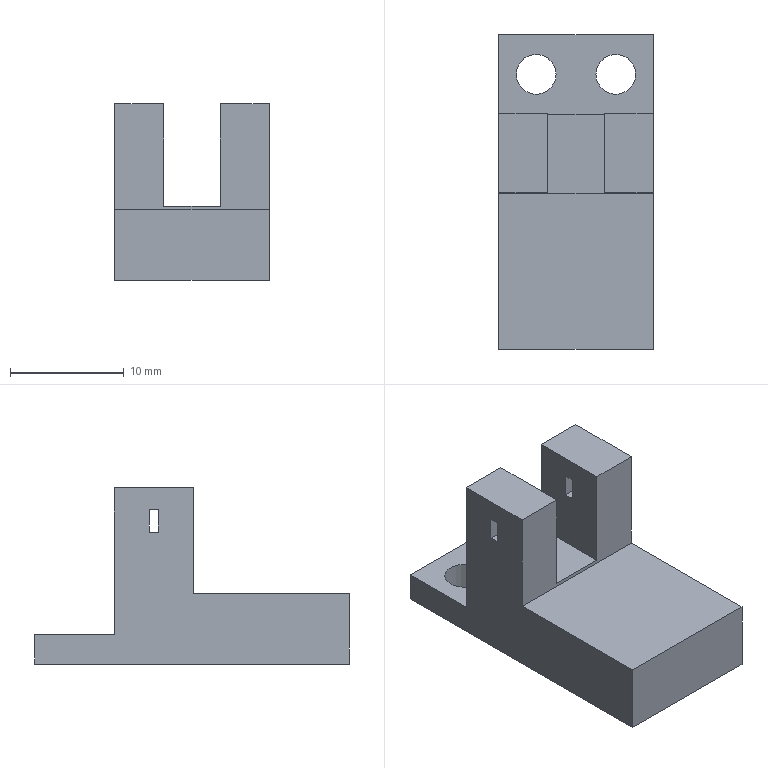Part | STEP file | 11-EE-SX674A11 | 1 solid | 26 faces | box 13.6 x 27.7 x 15.5 mm | volume 2495 mm3 | plane 22 | cylinder 4 | commonest cylinder face diameters 3.5 x4
STEP:
#1=CARTESIAN_POINT('',(12.05,24.2,0.));
#2=VERTEX_POINT('',#1);
#3=CARTESIAN_POINT('',(8.55,24.2,0.));
#4=VERTEX_POINT('',#3);
#5=CARTESIAN_POINT('',(10.3,24.2,0.));
#6=DIRECTION('',(0.,0.,-1.));
#7=DIRECTION('',(-1.,0.,0.));
#8=AXIS2_PLACEMENT_3D('',#5,#6,#7);
#9=CIRCLE('',#8,1.75);
#10=EDGE_CURVE('',#2,#4,#9,.T.);
#11=ORIENTED_EDGE('',*,*,#10,.T.);
#12=CARTESIAN_POINT('',(8.55,24.2,2.6));
#13=VERTEX_POINT('',#12);
#14=CARTESIAN_POINT('',(8.55,24.2,2.6));
#15=DIRECTION('',(0.,0.,1.));
#16=VECTOR('',#15,1000.);
#17=LINE('',#14,#16);
#18=EDGE_CURVE('',#4,#13,#17,.T.);
#19=ORIENTED_EDGE('',*,*,#18,.T.);
#20=CARTESIAN_POINT('',(12.05,24.2,2.6));
#21=VERTEX_POINT('',#20);
#22=CARTESIAN_POINT('',(10.3,24.2,2.6));
#23=DIRECTION('',(0.,0.,1.));
#24=DIRECTION('',(1.,0.,0.));
#25=AXIS2_PLACEMENT_3D('',#22,#23,#24);
#26=CIRCLE('',#25,1.75);
#27=EDGE_CURVE('',#13,#21,#26,.T.);
#28=ORIENTED_EDGE('',*,*,#27,.T.);
#29=CARTESIAN_POINT('',(12.05,24.2,2.6));
#30=DIRECTION('',(0.,0.,1.));
#31=VECTOR('',#30,1000.);
#32=LINE('',#29,#31);
#33=EDGE_CURVE('',#2,#21,#32,.T.);
#34=ORIENTED_EDGE('',*,*,#33,.F.);
#35=EDGE_LOOP('',(#11,#19,#28,#34));
#36=FACE_OUTER_BOUND('',#35,.T.);
#37=CARTESIAN_POINT('',(10.3,24.2,2.6));
#38=DIRECTION('',(0.,0.,1.));
#39=DIRECTION('',(1.,0.,0.));
#40=AXIS2_PLACEMENT_3D('',#37,#38,#39);
#41=CYLINDRICAL_SURFACE('',#40,1.75);
#42=ADVANCED_FACE('',(#36),#41,.F.);
#43=CARTESIAN_POINT('',(5.05,24.2,0.));
#44=VERTEX_POINT('',#43);
#45=CARTESIAN_POINT('',(1.55,24.2,0.));
#46=VERTEX_POINT('',#45);
#47=CARTESIAN_POINT('',(3.3,24.2,0.));
#48=DIRECTION('',(0.,0.,-1.));
#49=DIRECTION('',(-1.,0.,0.));
#50=AXIS2_PLACEMENT_3D('',#47,#48,#49);
#51=CIRCLE('',#50,1.75);
#52=EDGE_CURVE('',#44,#46,#51,.T.);
#53=ORIENTED_EDGE('',*,*,#52,.T.);
#54=CARTESIAN_POINT('',(1.55,24.2,2.6));
#55=VERTEX_POINT('',#54);
#56=CARTESIAN_POINT('',(1.55,24.2,2.6));
#57=DIRECTION('',(0.,0.,1.));
#58=VECTOR('',#57,1000.);
#59=LINE('',#56,#58);
#60=EDGE_CURVE('',#46,#55,#59,.T.);
#61=ORIENTED_EDGE('',*,*,#60,.T.);
#62=CARTESIAN_POINT('',(5.05,24.2,2.6));
#63=VERTEX_POINT('',#62);
#64=CARTESIAN_POINT('',(3.3,24.2,2.6));
#65=DIRECTION('',(0.,0.,1.));
#66=DIRECTION('',(1.,0.,0.));
#67=AXIS2_PLACEMENT_3D('',#64,#65,#66);
#68=CIRCLE('',#67,1.75);
#69=EDGE_CURVE('',#55,#63,#68,.T.);
#70=ORIENTED_EDGE('',*,*,#69,.T.);
#71=CARTESIAN_POINT('',(5.05,24.2,2.6));
#72=DIRECTION('',(0.,0.,1.));
#73=VECTOR('',#72,1000.);
#74=LINE('',#71,#73);
#75=EDGE_CURVE('',#44,#63,#74,.T.);
#76=ORIENTED_EDGE('',*,*,#75,.F.);
#77=EDGE_LOOP('',(#53,#61,#70,#76));
#78=FACE_OUTER_BOUND('',#77,.T.);
#79=CARTESIAN_POINT('',(3.3,24.2,2.6));
#80=DIRECTION('',(0.,0.,1.));
#81=DIRECTION('',(1.,0.,0.));
#82=AXIS2_PLACEMENT_3D('',#79,#80,#81);
#83=CYLINDRICAL_SURFACE('',#82,1.75);
#84=ADVANCED_FACE('',(#78),#83,.F.);
#85=CARTESIAN_POINT('',(0.,13.75,15.5));
#86=VERTEX_POINT('',#85);
#87=CARTESIAN_POINT('',(4.3,13.75,15.5));
#88=VERTEX_POINT('',#87);
#89=CARTESIAN_POINT('',(0.,13.75,15.5));
#90=DIRECTION('',(1.,0.,0.));
#91=VECTOR('',#90,1000.);
#92=LINE('',#89,#91);
#93=EDGE_CURVE('',#86,#88,#92,.T.);
#94=ORIENTED_EDGE('',*,*,#93,.T.);
#95=CARTESIAN_POINT('',(4.3,20.7,15.5));
#96=VERTEX_POINT('',#95);
#97=CARTESIAN_POINT('',(4.3,27.7,15.5));
#98=DIRECTION('',(0.,1.,0.));
#99=VECTOR('',#98,1000.);
#100=LINE('',#97,#99);
#101=EDGE_CURVE('',#88,#96,#100,.T.);
#102=ORIENTED_EDGE('',*,*,#101,.T.);
#103=CARTESIAN_POINT('',(0.,20.7,15.5));
#104=VERTEX_POINT('',#103);
#105=CARTESIAN_POINT('',(0.,20.7,15.5));
#106=DIRECTION('',(-1.,0.,0.));
#107=VECTOR('',#106,1000.);
#108=LINE('',#105,#107);
#109=EDGE_CURVE('',#96,#104,#108,.T.);
#110=ORIENTED_EDGE('',*,*,#109,.T.);
#111=CARTESIAN_POINT('',(0.,0.,15.5));
#112=DIRECTION('',(0.,-1.,0.));
#113=VECTOR('',#112,1000.);
#114=LINE('',#111,#113);
#115=EDGE_CURVE('',#104,#86,#114,.T.);
#116=ORIENTED_EDGE('',*,*,#115,.T.);
#117=EDGE_LOOP('',(#94,#102,#110,#116));
#118=FACE_OUTER_BOUND('',#117,.T.);
#119=CARTESIAN_POINT('',(0.,27.7,15.5));
#120=DIRECTION('',(0.,0.,-1.));
#121=DIRECTION('',(-1.,0.,0.));
#122=AXIS2_PLACEMENT_3D('',#119,#120,#121);
#123=PLANE('',#122);
#124=ADVANCED_FACE('',(#118),#123,.F.);
#125=CARTESIAN_POINT('',(0.,17.625,11.6));
#126=VERTEX_POINT('',#125);
#127=CARTESIAN_POINT('',(0.,17.625,13.6));
#128=VERTEX_POINT('',#127);
#129=CARTESIAN_POINT('',(0.,17.625,13.6));
#130=DIRECTION('',(0.,0.,1.));
#131=VECTOR('',#130,1000.);
#132=LINE('',#129,#131);
#133=EDGE_CURVE('',#126,#128,#132,.T.);
#134=ORIENTED_EDGE('',*,*,#133,.T.);
#135=CARTESIAN_POINT('',(0.,16.825,13.6));
#136=VERTEX_POINT('',#135);
#137=CARTESIAN_POINT('',(0.,17.625,13.6));
#138=DIRECTION('',(0.,-1.,0.));
#139=VECTOR('',#138,1000.);
#140=LINE('',#137,#139);
#141=EDGE_CURVE('',#128,#136,#140,.T.);
#142=ORIENTED_EDGE('',*,*,#141,.T.);
#143=CARTESIAN_POINT('',(0.,16.825,11.6));
#144=VERTEX_POINT('',#143);
#145=CARTESIAN_POINT('',(0.,16.825,13.6));
#146=DIRECTION('',(0.,0.,-1.));
#147=VECTOR('',#146,1000.);
#148=LINE('',#145,#147);
#149=EDGE_CURVE('',#136,#144,#148,.T.);
#150=ORIENTED_EDGE('',*,*,#149,.T.);
#151=CARTESIAN_POINT('',(0.,17.625,11.6));
#152=DIRECTION('',(0.,1.,0.));
#153=VECTOR('',#152,1000.);
#154=LINE('',#151,#153);
#155=EDGE_CURVE('',#144,#126,#154,.T.);
#156=ORIENTED_EDGE('',*,*,#155,.T.);
#157=EDGE_LOOP('',(#134,#142,#150,#156));
#158=FACE_BOUND('',#157,.T.);
#159=CARTESIAN_POINT('',(0.,0.,6.2));
#160=VERTEX_POINT('',#159);
#161=CARTESIAN_POINT('',(0.,13.75,6.2));
#162=VERTEX_POINT('',#161);
#163=CARTESIAN_POINT('',(0.,13.75,6.2));
#164=DIRECTION('',(0.,1.,0.));
#165=VECTOR('',#164,1000.);
#166=LINE('',#163,#165);
#167=EDGE_CURVE('',#160,#162,#166,.T.);
#168=ORIENTED_EDGE('',*,*,#167,.T.);
#169=CARTESIAN_POINT('',(0.,13.75,21.475));
#170=DIRECTION('',(0.,0.,1.));
#171=VECTOR('',#170,1000.);
#172=LINE('',#169,#171);
#173=EDGE_CURVE('',#162,#86,#172,.T.);
#174=ORIENTED_EDGE('',*,*,#173,.T.);
#175=ORIENTED_EDGE('',*,*,#115,.F.);
#176=CARTESIAN_POINT('',(0.,20.7,2.6));
#177=VERTEX_POINT('',#176);
#178=CARTESIAN_POINT('',(0.,20.7,18.769));
#179=DIRECTION('',(0.,0.,-1.));
#180=VECTOR('',#179,1000.);
#181=LINE('',#178,#180);
#182=EDGE_CURVE('',#104,#177,#181,.T.);
#183=ORIENTED_EDGE('',*,*,#182,.T.);
#184=CARTESIAN_POINT('',(0.,27.7,2.6));
#185=VERTEX_POINT('',#184);
#186=CARTESIAN_POINT('',(0.,31.417,2.6));
#187=DIRECTION('',(0.,1.,0.));
#188=VECTOR('',#187,1000.);
#189=LINE('',#186,#188);
#190=EDGE_CURVE('',#177,#185,#189,.T.);
#191=ORIENTED_EDGE('',*,*,#190,.T.);
#192=CARTESIAN_POINT('',(0.,27.7,0.));
#193=VERTEX_POINT('',#192);
#194=CARTESIAN_POINT('',(0.,27.7,15.5));
#195=DIRECTION('',(0.,0.,-1.));
#196=VECTOR('',#195,1000.);
#197=LINE('',#194,#196);
#198=EDGE_CURVE('',#185,#193,#197,.T.);
#199=ORIENTED_EDGE('',*,*,#198,.T.);
#200=CARTESIAN_POINT('',(0.,0.,0.));
#201=VERTEX_POINT('',#200);
#202=CARTESIAN_POINT('',(0.,0.,0.));
#203=DIRECTION('',(0.,-1.,0.));
#204=VECTOR('',#203,1000.);
#205=LINE('',#202,#204);
#206=EDGE_CURVE('',#193,#201,#205,.T.);
#207=ORIENTED_EDGE('',*,*,#206,.T.);
#208=CARTESIAN_POINT('',(0.,0.,15.5));
#209=DIRECTION('',(0.,0.,-1.));
#210=VECTOR('',#209,1000.);
#211=LINE('',#208,#210);
#212=EDGE_CURVE('',#160,#201,#211,.T.);
#213=ORIENTED_EDGE('',*,*,#212,.F.);
#214=EDGE_LOOP('',(#168,#174,#175,#183,#191,#199,#207,#213));
#215=FACE_OUTER_BOUND('',#214,.T.);
#216=CARTESIAN_POINT('',(0.,0.,15.5));
#217=DIRECTION('',(1.,0.,0.));
#218=DIRECTION('',(0.,0.,-1.));
#219=AXIS2_PLACEMENT_3D('',#216,#217,#218);
#220=PLANE('',#219);
#221=ADVANCED_FACE('',(#158,#215),#220,.F.);
#222=CARTESIAN_POINT('',(13.6,0.,6.2));
#223=VERTEX_POINT('',#222);
#224=CARTESIAN_POINT('',(13.6,0.,0.));
#225=VERTEX_POINT('',#224);
#226=CARTESIAN_POINT('',(13.6,0.,15.5));
#227=DIRECTION('',(0.,0.,-1.));
#228=VECTOR('',#227,1000.);
#229=LINE('',#226,#228);
#230=EDGE_CURVE('',#223,#225,#229,.T.);
#231=ORIENTED_EDGE('',*,*,#230,.F.);
#232=CARTESIAN_POINT('',(0.,0.,6.2));
#233=DIRECTION('',(-1.,0.,0.));
#234=VECTOR('',#233,1000.);
#235=LINE('',#232,#234);
#236=EDGE_CURVE('',#223,#160,#235,.T.);
#237=ORIENTED_EDGE('',*,*,#236,.T.);
#238=ORIENTED_EDGE('',*,*,#212,.T.);
#239=CARTESIAN_POINT('',(0.,0.,0.));
#240=DIRECTION('',(1.,0.,0.));
#241=VECTOR('',#240,1000.);
#242=LINE('',#239,#241);
#243=EDGE_CURVE('',#201,#225,#242,.T.);
#244=ORIENTED_EDGE('',*,*,#243,.T.);
#245=EDGE_LOOP('',(#231,#237,#238,#244));
#246=FACE_OUTER_BOUND('',#245,.T.);
#247=CARTESIAN_POINT('',(0.,0.,15.5));
#248=DIRECTION('',(0.,1.,0.));
#249=DIRECTION('',(0.,0.,1.));
#250=AXIS2_PLACEMENT_3D('',#247,#248,#249);
#251=PLANE('',#250);
#252=ADVANCED_FACE('',(#246),#251,.F.);
#253=CARTESIAN_POINT('',(13.6,16.825,13.6));
#254=VERTEX_POINT('',#253);
#255=CARTESIAN_POINT('',(13.6,16.825,11.6));
#256=VERTEX_POINT('',#255);
#257=CARTESIAN_POINT('',(13.6,16.825,13.6));
#258=DIRECTION('',(0.,0.,-1.));
#259=VECTOR('',#258,1000.);
#260=LINE('',#257,#259);
#261=EDGE_CURVE('',#254,#256,#260,.T.);
#262=ORIENTED_EDGE('',*,*,#261,.F.);
#263=CARTESIAN_POINT('',(13.6,17.625,13.6));
#264=VERTEX_POINT('',#263);
#265=CARTESIAN_POINT('',(13.6,17.625,13.6));
#266=DIRECTION('',(0.,-1.,0.));
#267=VECTOR('',#266,1000.);
#268=LINE('',#265,#267);
#269=EDGE_CURVE('',#264,#254,#268,.T.);
#270=ORIENTED_EDGE('',*,*,#269,.F.);
#271=CARTESIAN_POINT('',(13.6,17.625,11.6));
#272=VERTEX_POINT('',#271);
#273=CARTESIAN_POINT('',(13.6,17.625,13.6));
#274=DIRECTION('',(0.,0.,1.));
#275=VECTOR('',#274,1000.);
#276=LINE('',#273,#275);
#277=EDGE_CURVE('',#272,#264,#276,.T.);
#278=ORIENTED_EDGE('',*,*,#277,.F.);
#279=CARTESIAN_POINT('',(13.6,17.625,11.6));
#280=DIRECTION('',(0.,1.,0.));
#281=VECTOR('',#280,1000.);
#282=LINE('',#279,#281);
#283=EDGE_CURVE('',#256,#272,#282,.T.);
#284=ORIENTED_EDGE('',*,*,#283,.F.);
#285=EDGE_LOOP('',(#262,#270,#278,#284));
#286=FACE_BOUND('',#285,.T.);
#287=CARTESIAN_POINT('',(13.6,13.75,15.5));
#288=VERTEX_POINT('',#287);
#289=CARTESIAN_POINT('',(13.6,20.7,15.5));
#290=VERTEX_POINT('',#289);
#291=CARTESIAN_POINT('',(13.6,0.,15.5));
#292=DIRECTION('',(0.,1.,0.));
#293=VECTOR('',#292,1000.);
#294=LINE('',#291,#293);
#295=EDGE_CURVE('',#288,#290,#294,.T.);
#296=ORIENTED_EDGE('',*,*,#295,.F.);
#297=CARTESIAN_POINT('',(13.6,13.75,6.2));
#298=VERTEX_POINT('',#297);
#299=CARTESIAN_POINT('',(13.6,13.75,21.475));
#300=DIRECTION('',(0.,0.,1.));
#301=VECTOR('',#300,1000.);
#302=LINE('',#299,#301);
#303=EDGE_CURVE('',#298,#288,#302,.T.);
#304=ORIENTED_EDGE('',*,*,#303,.F.);
#305=CARTESIAN_POINT('',(13.6,13.75,6.2));
#306=DIRECTION('',(0.,1.,0.));
#307=VECTOR('',#306,1000.);
#308=LINE('',#305,#307);
#309=EDGE_CURVE('',#223,#298,#308,.T.);
#310=ORIENTED_EDGE('',*,*,#309,.F.);
#311=ORIENTED_EDGE('',*,*,#230,.T.);
#312=CARTESIAN_POINT('',(13.6,27.7,0.));
#313=VERTEX_POINT('',#312);
#314=CARTESIAN_POINT('',(13.6,0.,0.));
#315=DIRECTION('',(0.,1.,0.));
#316=VECTOR('',#315,1000.);
#317=LINE('',#314,#316);
#318=EDGE_CURVE('',#225,#313,#317,.T.);
#319=ORIENTED_EDGE('',*,*,#318,.T.);
#320=CARTESIAN_POINT('',(13.6,27.7,2.6));
#321=VERTEX_POINT('',#320);
#322=CARTESIAN_POINT('',(13.6,27.7,15.5));
#323=DIRECTION('',(0.,0.,-1.));
#324=VECTOR('',#323,1000.);
#325=LINE('',#322,#324);
#326=EDGE_CURVE('',#321,#313,#325,.T.);
#327=ORIENTED_EDGE('',*,*,#326,.F.);
#328=CARTESIAN_POINT('',(13.6,20.7,2.6));
#329=VERTEX_POINT('',#328);
#330=CARTESIAN_POINT('',(13.6,31.417,2.6));
#331=DIRECTION('',(0.,1.,0.));
#332=VECTOR('',#331,1000.);
#333=LINE('',#330,#332);
#334=EDGE_CURVE('',#329,#321,#333,.T.);
#335=ORIENTED_EDGE('',*,*,#334,.F.);
#336=CARTESIAN_POINT('',(13.6,20.7,18.769));
#337=DIRECTION('',(0.,0.,-1.));
#338=VECTOR('',#337,1000.);
#339=LINE('',#336,#338);
#340=EDGE_CURVE('',#290,#329,#339,.T.);
#341=ORIENTED_EDGE('',*,*,#340,.F.);
#342=EDGE_LOOP('',(#296,#304,#310,#311,#319,#327,#335,#341));
#343=FACE_OUTER_BOUND('',#342,.T.);
#344=CARTESIAN_POINT('',(13.6,0.,15.5));
#345=DIRECTION('',(-1.,0.,0.));
#346=DIRECTION('',(0.,0.,1.));
#347=AXIS2_PLACEMENT_3D('',#344,#345,#346);
#348=PLANE('',#347);
#349=ADVANCED_FACE('',(#286,#343),#348,.F.);
#350=ORIENTED_EDGE('',*,*,#198,.F.);
#351=CARTESIAN_POINT('',(0.,27.7,2.6));
#352=DIRECTION('',(1.,0.,0.));
#353=VECTOR('',#352,1000.);
#354=LINE('',#351,#353);
#355=EDGE_CURVE('',#185,#321,#354,.T.);
#356=ORIENTED_EDGE('',*,*,#355,.T.);
#357=ORIENTED_EDGE('',*,*,#326,.T.);
#358=CARTESIAN_POINT('',(0.,27.7,0.));
#359=DIRECTION('',(-1.,0.,0.));
#360=VECTOR('',#359,1000.);
#361=LINE('',#358,#360);
#362=EDGE_CURVE('',#313,#193,#361,.T.);
#363=ORIENTED_EDGE('',*,*,#362,.T.);
#364=EDGE_LOOP('',(#350,#356,#357,#363));
#365=FACE_OUTER_BOUND('',#364,.T.);
#366=CARTESIAN_POINT('',(0.,27.7,15.5));
#367=DIRECTION('',(0.,-1.,0.));
#368=DIRECTION('',(0.,0.,-1.));
#369=AXIS2_PLACEMENT_3D('',#366,#367,#368);
#370=PLANE('',#369);
#371=ADVANCED_FACE('',(#365),#370,.F.);
#372=CARTESIAN_POINT('',(9.3,20.7,15.5));
#373=VERTEX_POINT('',#372);
#374=CARTESIAN_POINT('',(0.,20.7,15.5));
#375=DIRECTION('',(-1.,0.,0.));
#376=VECTOR('',#375,1000.);
#377=LINE('',#374,#376);
#378=EDGE_CURVE('',#290,#373,#377,.T.);
#379=ORIENTED_EDGE('',*,*,#378,.T.);
#380=CARTESIAN_POINT('',(9.3,13.75,15.5));
#381=VERTEX_POINT('',#380);
#382=CARTESIAN_POINT('',(9.3,27.7,15.5));
#383=DIRECTION('',(0.,-1.,0.));
#384=VECTOR('',#383,1000.);
#385=LINE('',#382,#384);
#386=EDGE_CURVE('',#373,#381,#385,.T.);
#387=ORIENTED_EDGE('',*,*,#386,.T.);
#388=CARTESIAN_POINT('',(0.,13.75,15.5));
#389=DIRECTION('',(1.,0.,0.));
#390=VECTOR('',#389,1000.);
#391=LINE('',#388,#390);
#392=EDGE_CURVE('',#381,#288,#391,.T.);
#393=ORIENTED_EDGE('',*,*,#392,.T.);
#394=ORIENTED_EDGE('',*,*,#295,.T.);
#395=EDGE_LOOP('',(#379,#387,#393,#394));
#396=FACE_OUTER_BOUND('',#395,.T.);
#397=CARTESIAN_POINT('',(0.,27.7,15.5));
#398=DIRECTION('',(0.,0.,-1.));
#399=DIRECTION('',(-1.,0.,0.));
#400=AXIS2_PLACEMENT_3D('',#397,#398,#399);
#401=PLANE('',#400);
#402=ADVANCED_FACE('',(#396),#401,.F.);
#403=ORIENTED_EDGE('',*,*,#10,.F.);
#404=CARTESIAN_POINT('',(10.3,24.2,0.));
#405=DIRECTION('',(0.,0.,-1.));
#406=DIRECTION('',(-1.,0.,0.));
#407=AXIS2_PLACEMENT_3D('',#404,#405,#406);
#408=CIRCLE('',#407,1.75);
#409=EDGE_CURVE('',#4,#2,#408,.T.);
#410=ORIENTED_EDGE('',*,*,#409,.F.);
#411=EDGE_LOOP('',(#403,#410));
#412=FACE_BOUND('',#411,.T.);
#413=ORIENTED_EDGE('',*,*,#52,.F.);
#414=CARTESIAN_POINT('',(3.3,24.2,0.));
#415=DIRECTION('',(0.,0.,-1.));
#416=DIRECTION('',(-1.,0.,0.));
#417=AXIS2_PLACEMENT_3D('',#414,#415,#416);
#418=CIRCLE('',#417,1.75);
#419=EDGE_CURVE('',#46,#44,#418,.T.);
#420=ORIENTED_EDGE('',*,*,#419,.F.);
#421=EDGE_LOOP('',(#413,#420));
#422=FACE_BOUND('',#421,.T.);
#423=ORIENTED_EDGE('',*,*,#206,.F.);
#424=ORIENTED_EDGE('',*,*,#362,.F.);
#425=ORIENTED_EDGE('',*,*,#318,.F.);
#426=ORIENTED_EDGE('',*,*,#243,.F.);
#427=EDGE_LOOP('',(#423,#424,#425,#426));
#428=FACE_OUTER_BOUND('',#427,.T.);
#429=CARTESIAN_POINT('',(0.,27.7,0.));
#430=DIRECTION('',(0.,0.,-1.));
#431=DIRECTION('',(-1.,0.,0.));
#432=AXIS2_PLACEMENT_3D('',#429,#430,#431);
#433=PLANE('',#432);
#434=ADVANCED_FACE('',(#412,#422,#428),#433,.T.);
#435=CARTESIAN_POINT('',(10.3,24.2,2.6));
#436=DIRECTION('',(0.,0.,1.));
#437=DIRECTION('',(1.,0.,0.));
#438=AXIS2_PLACEMENT_3D('',#435,#436,#437);
#439=CIRCLE('',#438,1.75);
#440=EDGE_CURVE('',#21,#13,#439,.T.);
#441=ORIENTED_EDGE('',*,*,#440,.F.);
#442=ORIENTED_EDGE('',*,*,#27,.F.);
#443=EDGE_LOOP('',(#441,#442));
#444=FACE_BOUND('',#443,.T.);
#445=CARTESIAN_POINT('',(3.3,24.2,2.6));
#446=DIRECTION('',(0.,0.,1.));
#447=DIRECTION('',(1.,0.,0.));
#448=AXIS2_PLACEMENT_3D('',#445,#446,#447);
#449=CIRCLE('',#448,1.75);
#450=EDGE_CURVE('',#63,#55,#449,.T.);
#451=ORIENTED_EDGE('',*,*,#450,.F.);
#452=ORIENTED_EDGE('',*,*,#69,.F.);
#453=EDGE_LOOP('',(#451,#452));
#454=FACE_BOUND('',#453,.T.);
#455=ORIENTED_EDGE('',*,*,#190,.F.);
#456=CARTESIAN_POINT('',(0.,20.7,2.6));
#457=DIRECTION('',(1.,0.,0.));
#458=VECTOR('',#457,1000.);
#459=LINE('',#456,#458);
#460=EDGE_CURVE('',#177,#329,#459,.T.);
#461=ORIENTED_EDGE('',*,*,#460,.T.);
#462=ORIENTED_EDGE('',*,*,#334,.T.);
#463=ORIENTED_EDGE('',*,*,#355,.F.);
#464=EDGE_LOOP('',(#455,#461,#462,#463));
#465=FACE_OUTER_BOUND('',#464,.T.);
#466=CARTESIAN_POINT('',(0.,31.417,2.6));
#467=DIRECTION('',(0.,0.,-1.));
#468=DIRECTION('',(0.,1.,0.));
#469=AXIS2_PLACEMENT_3D('',#466,#467,#468);
#470=PLANE('',#469);
#471=ADVANCED_FACE('',(#444,#454,#465),#470,.F.);
#472=ORIENTED_EDGE('',*,*,#109,.F.);
#473=CARTESIAN_POINT('',(4.3,20.7,6.5));
#474=VERTEX_POINT('',#473);
#475=CARTESIAN_POINT('',(4.3,20.7,18.769));
#476=DIRECTION('',(0.,0.,-1.));
#477=VECTOR('',#476,1000.);
#478=LINE('',#475,#477);
#479=EDGE_CURVE('',#96,#474,#478,.T.);
#480=ORIENTED_EDGE('',*,*,#479,.T.);
#481=CARTESIAN_POINT('',(9.3,20.7,6.5));
#482=VERTEX_POINT('',#481);
#483=CARTESIAN_POINT('',(0.,20.7,6.5));
#484=DIRECTION('',(1.,0.,0.));
#485=VECTOR('',#484,1000.);
#486=LINE('',#483,#485);
#487=EDGE_CURVE('',#474,#482,#486,.T.);
#488=ORIENTED_EDGE('',*,*,#487,.T.);
#489=CARTESIAN_POINT('',(9.3,20.7,18.769));
#490=DIRECTION('',(0.,0.,1.));
#491=VECTOR('',#490,1000.);
#492=LINE('',#489,#491);
#493=EDGE_CURVE('',#482,#373,#492,.T.);
#494=ORIENTED_EDGE('',*,*,#493,.T.);
#495=ORIENTED_EDGE('',*,*,#378,.F.);
#496=ORIENTED_EDGE('',*,*,#340,.T.);
#497=ORIENTED_EDGE('',*,*,#460,.F.);
#498=ORIENTED_EDGE('',*,*,#182,.F.);
#499=EDGE_LOOP('',(#472,#480,#488,#494,#495,#496,#497,#498));
#500=FACE_OUTER_BOUND('',#499,.T.);
#501=CARTESIAN_POINT('',(0.,20.7,18.769));
#502=DIRECTION('',(0.,-1.,0.));
#503=DIRECTION('',(0.,0.,-1.));
#504=AXIS2_PLACEMENT_3D('',#501,#502,#503);
#505=PLANE('',#504);
#506=ADVANCED_FACE('',(#500),#505,.F.);
#507=ORIENTED_EDGE('',*,*,#309,.T.);
#508=CARTESIAN_POINT('',(0.,13.75,6.2));
#509=DIRECTION('',(1.,0.,0.));
#510=VECTOR('',#509,1000.);
#511=LINE('',#508,#510);
#512=EDGE_CURVE('',#162,#298,#511,.T.);
#513=ORIENTED_EDGE('',*,*,#512,.F.);
#514=ORIENTED_EDGE('',*,*,#167,.F.);
#515=ORIENTED_EDGE('',*,*,#236,.F.);
#516=EDGE_LOOP('',(#507,#513,#514,#515));
#517=FACE_OUTER_BOUND('',#516,.T.);
#518=CARTESIAN_POINT('',(0.,13.75,6.2));
#519=DIRECTION('',(0.,0.,-1.));
#520=DIRECTION('',(0.,1.,0.));
#521=AXIS2_PLACEMENT_3D('',#518,#519,#520);
#522=PLANE('',#521);
#523=ADVANCED_FACE('',(#517),#522,.F.);
#524=CARTESIAN_POINT('',(9.3,13.75,6.5));
#525=VERTEX_POINT('',#524);
#526=CARTESIAN_POINT('',(4.3,13.75,6.5));
#527=VERTEX_POINT('',#526);
#528=CARTESIAN_POINT('',(0.,13.75,6.5));
#529=DIRECTION('',(-1.,0.,0.));
#530=VECTOR('',#529,1000.);
#531=LINE('',#528,#530);
#532=EDGE_CURVE('',#525,#527,#531,.T.);
#533=ORIENTED_EDGE('',*,*,#532,.T.);
#534=CARTESIAN_POINT('',(4.3,13.75,21.475));
#535=DIRECTION('',(0.,0.,1.));
#536=VECTOR('',#535,1000.);
#537=LINE('',#534,#536);
#538=EDGE_CURVE('',#527,#88,#537,.T.);
#539=ORIENTED_EDGE('',*,*,#538,.T.);
#540=ORIENTED_EDGE('',*,*,#93,.F.);
#541=ORIENTED_EDGE('',*,*,#173,.F.);
#542=ORIENTED_EDGE('',*,*,#512,.T.);
#543=ORIENTED_EDGE('',*,*,#303,.T.);
#544=ORIENTED_EDGE('',*,*,#392,.F.);
#545=CARTESIAN_POINT('',(9.3,13.75,21.475));
#546=DIRECTION('',(0.,0.,-1.));
#547=VECTOR('',#546,1000.);
#548=LINE('',#545,#547);
#549=EDGE_CURVE('',#381,#525,#548,.T.);
#550=ORIENTED_EDGE('',*,*,#549,.T.);
#551=EDGE_LOOP('',(#533,#539,#540,#541,#542,#543,#544,#550));
#552=FACE_OUTER_BOUND('',#551,.T.);
#553=CARTESIAN_POINT('',(0.,13.75,21.475));
#554=DIRECTION('',(0.,1.,0.));
#555=DIRECTION('',(0.,0.,1.));
#556=AXIS2_PLACEMENT_3D('',#553,#554,#555);
#557=PLANE('',#556);
#558=ADVANCED_FACE('',(#552),#557,.F.);
#559=CARTESIAN_POINT('',(4.3,16.825,11.6));
#560=VERTEX_POINT('',#559);
#561=CARTESIAN_POINT('',(4.3,16.825,13.6));
#562=VERTEX_POINT('',#561);
#563=CARTESIAN_POINT('',(4.3,16.825,17.591));
#564=DIRECTION('',(0.,0.,1.));
#565=VECTOR('',#564,1000.);
#566=LINE('',#563,#565);
#567=EDGE_CURVE('',#560,#562,#566,.T.);
#568=ORIENTED_EDGE('',*,*,#567,.T.);
#569=CARTESIAN_POINT('',(4.3,17.625,13.6));
#570=VERTEX_POINT('',#569);
#571=CARTESIAN_POINT('',(4.3,27.7,13.6));
#572=DIRECTION('',(0.,1.,0.));
#573=VECTOR('',#572,1000.);
#574=LINE('',#571,#573);
#575=EDGE_CURVE('',#562,#570,#574,.T.);
#576=ORIENTED_EDGE('',*,*,#575,.T.);
#577=CARTESIAN_POINT('',(4.3,17.625,11.6));
#578=VERTEX_POINT('',#577);
#579=CARTESIAN_POINT('',(4.3,17.625,17.591));
#580=DIRECTION('',(0.,0.,-1.));
#581=VECTOR('',#580,1000.);
#582=LINE('',#579,#581);
#583=EDGE_CURVE('',#570,#578,#582,.T.);
#584=ORIENTED_EDGE('',*,*,#583,.T.);
#585=CARTESIAN_POINT('',(4.3,27.7,11.6));
#586=DIRECTION('',(0.,-1.,0.));
#587=VECTOR('',#586,1000.);
#588=LINE('',#585,#587);
#589=EDGE_CURVE('',#578,#560,#588,.T.);
#590=ORIENTED_EDGE('',*,*,#589,.T.);
#591=EDGE_LOOP('',(#568,#576,#584,#590));
#592=FACE_BOUND('',#591,.T.);
#593=ORIENTED_EDGE('',*,*,#101,.F.);
#594=ORIENTED_EDGE('',*,*,#538,.F.);
#595=CARTESIAN_POINT('',(4.3,27.7,6.5));
#596=DIRECTION('',(0.,-1.,0.));
#597=VECTOR('',#596,1000.);
#598=LINE('',#595,#597);
#599=EDGE_CURVE('',#474,#527,#598,.T.);
#600=ORIENTED_EDGE('',*,*,#599,.F.);
#601=ORIENTED_EDGE('',*,*,#479,.F.);
#602=EDGE_LOOP('',(#593,#594,#600,#601));
#603=FACE_OUTER_BOUND('',#602,.T.);
#604=CARTESIAN_POINT('',(4.3,27.7,17.591));
#605=DIRECTION('',(-1.,0.,0.));
#606=DIRECTION('',(0.,0.,1.));
#607=AXIS2_PLACEMENT_3D('',#604,#605,#606);
#608=PLANE('',#607);
#609=ADVANCED_FACE('',(#592,#603),#608,.F.);
#610=CARTESIAN_POINT('',(9.3,17.625,11.6));
#611=VERTEX_POINT('',#610);
#612=CARTESIAN_POINT('',(9.3,17.625,13.6));
#613=VERTEX_POINT('',#612);
#614=CARTESIAN_POINT('',(9.3,17.625,17.591));
#615=DIRECTION('',(0.,0.,1.));
#616=VECTOR('',#615,1000.);
#617=LINE('',#614,#616);
#618=EDGE_CURVE('',#611,#613,#617,.T.);
#619=ORIENTED_EDGE('',*,*,#618,.T.);
#620=CARTESIAN_POINT('',(9.3,16.825,13.6));
#621=VERTEX_POINT('',#620);
#622=CARTESIAN_POINT('',(9.3,27.7,13.6));
#623=DIRECTION('',(0.,-1.,0.));
#624=VECTOR('',#623,1000.);
#625=LINE('',#622,#624);
#626=EDGE_CURVE('',#613,#621,#625,.T.);
#627=ORIENTED_EDGE('',*,*,#626,.T.);
#628=CARTESIAN_POINT('',(9.3,16.825,11.6));
#629=VERTEX_POINT('',#628);
#630=CARTESIAN_POINT('',(9.3,16.825,17.591));
#631=DIRECTION('',(0.,0.,-1.));
#632=VECTOR('',#631,1000.);
#633=LINE('',#630,#632);
#634=EDGE_CURVE('',#621,#629,#633,.T.);
#635=ORIENTED_EDGE('',*,*,#634,.T.);
#636=CARTESIAN_POINT('',(9.3,27.7,11.6));
#637=DIRECTION('',(0.,1.,0.));
#638=VECTOR('',#637,1000.);
#639=LINE('',#636,#638);
#640=EDGE_CURVE('',#629,#611,#639,.T.);
#641=ORIENTED_EDGE('',*,*,#640,.T.);
#642=EDGE_LOOP('',(#619,#627,#635,#641));
#643=FACE_BOUND('',#642,.T.);
#644=CARTESIAN_POINT('',(9.3,27.7,6.5));
#645=DIRECTION('',(0.,-1.,0.));
#646=VECTOR('',#645,1000.);
#647=LINE('',#644,#646);
#648=EDGE_CURVE('',#482,#525,#647,.T.);
#649=ORIENTED_EDGE('',*,*,#648,.T.);
#650=ORIENTED_EDGE('',*,*,#549,.F.);
#651=ORIENTED_EDGE('',*,*,#386,.F.);
#652=ORIENTED_EDGE('',*,*,#493,.F.);
#653=EDGE_LOOP('',(#649,#650,#651,#652));
#654=FACE_OUTER_BOUND('',#653,.T.);
#655=CARTESIAN_POINT('',(9.3,27.7,17.591));
#656=DIRECTION('',(1.,0.,0.));
#657=DIRECTION('',(0.,0.,-1.));
#658=AXIS2_PLACEMENT_3D('',#655,#656,#657);
#659=PLANE('',#658);
#660=ADVANCED_FACE('',(#643,#654),#659,.F.);
#661=ORIENTED_EDGE('',*,*,#599,.T.);
#662=ORIENTED_EDGE('',*,*,#532,.F.);
#663=ORIENTED_EDGE('',*,*,#648,.F.);
#664=ORIENTED_EDGE('',*,*,#487,.F.);
#665=EDGE_LOOP('',(#661,#662,#663,#664));
#666=FACE_OUTER_BOUND('',#665,.T.);
#667=CARTESIAN_POINT('',(4.3,27.7,6.5));
#668=DIRECTION('',(0.,0.,-1.));
#669=DIRECTION('',(-1.,0.,0.));
#670=AXIS2_PLACEMENT_3D('',#667,#668,#669);
#671=PLANE('',#670);
#672=ADVANCED_FACE('',(#666),#671,.F.);
#673=CARTESIAN_POINT('',(0.,16.825,13.6));
#674=DIRECTION('',(1.,0.,0.));
#675=VECTOR('',#674,1000.);
#676=LINE('',#673,#675);
#677=EDGE_CURVE('',#621,#254,#676,.T.);
#678=ORIENTED_EDGE('',*,*,#677,.T.);
#679=ORIENTED_EDGE('',*,*,#261,.T.);
#680=CARTESIAN_POINT('',(0.,16.825,11.6));
#681=DIRECTION('',(1.,0.,0.));
#682=VECTOR('',#681,1000.);
#683=LINE('',#680,#682);
#684=EDGE_CURVE('',#629,#256,#683,.T.);
#685=ORIENTED_EDGE('',*,*,#684,.F.);
#686=ORIENTED_EDGE('',*,*,#634,.F.);
#687=EDGE_LOOP('',(#678,#679,#685,#686));
#688=FACE_OUTER_BOUND('',#687,.T.);
#689=CARTESIAN_POINT('',(0.,16.825,13.6));
#690=DIRECTION('',(0.,-1.,0.));
#691=DIRECTION('',(0.,0.,-1.));
#692=AXIS2_PLACEMENT_3D('',#689,#690,#691);
#693=PLANE('',#692);
#694=ADVANCED_FACE('',(#688),#693,.F.);
#695=ORIENTED_EDGE('',*,*,#684,.T.);
#696=ORIENTED_EDGE('',*,*,#283,.T.);
#697=CARTESIAN_POINT('',(0.,17.625,11.6));
#698=DIRECTION('',(1.,0.,0.));
#699=VECTOR('',#698,1000.);
#700=LINE('',#697,#699);
#701=EDGE_CURVE('',#611,#272,#700,.T.);
#702=ORIENTED_EDGE('',*,*,#701,.F.);
#703=ORIENTED_EDGE('',*,*,#640,.F.);
#704=EDGE_LOOP('',(#695,#696,#702,#703));
#705=FACE_OUTER_BOUND('',#704,.T.);
#706=CARTESIAN_POINT('',(0.,17.625,11.6));
#707=DIRECTION('',(0.,0.,-1.));
#708=DIRECTION('',(-1.,0.,0.));
#709=AXIS2_PLACEMENT_3D('',#706,#707,#708);
#710=PLANE('',#709);
#711=ADVANCED_FACE('',(#705),#710,.F.);
#712=ORIENTED_EDGE('',*,*,#701,.T.);
#713=ORIENTED_EDGE('',*,*,#277,.T.);
#714=CARTESIAN_POINT('',(0.,17.625,13.6));
#715=DIRECTION('',(1.,0.,0.));
#716=VECTOR('',#715,1000.);
#717=LINE('',#714,#716);
#718=EDGE_CURVE('',#613,#264,#717,.T.);
#719=ORIENTED_EDGE('',*,*,#718,.F.);
#720=ORIENTED_EDGE('',*,*,#618,.F.);
#721=EDGE_LOOP('',(#712,#713,#719,#720));
#722=FACE_OUTER_BOUND('',#721,.T.);
#723=CARTESIAN_POINT('',(0.,17.625,13.6));
#724=DIRECTION('',(0.,1.,0.));
#725=DIRECTION('',(0.,0.,1.));
#726=AXIS2_PLACEMENT_3D('',#723,#724,#725);
#727=PLANE('',#726);
#728=ADVANCED_FACE('',(#722),#727,.F.);
#729=ORIENTED_EDGE('',*,*,#718,.T.);
#730=ORIENTED_EDGE('',*,*,#269,.T.);
#731=ORIENTED_EDGE('',*,*,#677,.F.);
#732=ORIENTED_EDGE('',*,*,#626,.F.);
#733=EDGE_LOOP('',(#729,#730,#731,#732));
#734=FACE_OUTER_BOUND('',#733,.T.);
#735=CARTESIAN_POINT('',(0.,17.625,13.6));
#736=DIRECTION('',(0.,0.,1.));
#737=DIRECTION('',(1.,0.,0.));
#738=AXIS2_PLACEMENT_3D('',#735,#736,#737);
#739=PLANE('',#738);
#740=ADVANCED_FACE('',(#734),#739,.F.);
#741=CARTESIAN_POINT('',(0.,16.825,13.6));
#742=DIRECTION('',(1.,0.,0.));
#743=VECTOR('',#742,1000.);
#744=LINE('',#741,#743);
#745=EDGE_CURVE('',#136,#562,#744,.T.);
#746=ORIENTED_EDGE('',*,*,#745,.F.);
#747=ORIENTED_EDGE('',*,*,#141,.F.);
#748=CARTESIAN_POINT('',(0.,17.625,13.6));
#749=DIRECTION('',(1.,0.,0.));
#750=VECTOR('',#749,1000.);
#751=LINE('',#748,#750);
#752=EDGE_CURVE('',#128,#570,#751,.T.);
#753=ORIENTED_EDGE('',*,*,#752,.T.);
#754=ORIENTED_EDGE('',*,*,#575,.F.);
#755=EDGE_LOOP('',(#746,#747,#753,#754));
#756=FACE_OUTER_BOUND('',#755,.T.);
#757=CARTESIAN_POINT('',(0.,17.625,13.6));
#758=DIRECTION('',(0.,0.,1.));
#759=DIRECTION('',(1.,0.,0.));
#760=AXIS2_PLACEMENT_3D('',#757,#758,#759);
#761=PLANE('',#760);
#762=ADVANCED_FACE('',(#756),#761,.F.);
#763=ORIENTED_EDGE('',*,*,#752,.F.);
#764=ORIENTED_EDGE('',*,*,#133,.F.);
#765=CARTESIAN_POINT('',(0.,17.625,11.6));
#766=DIRECTION('',(1.,0.,0.));
#767=VECTOR('',#766,1000.);
#768=LINE('',#765,#767);
#769=EDGE_CURVE('',#126,#578,#768,.T.);
#770=ORIENTED_EDGE('',*,*,#769,.T.);
#771=ORIENTED_EDGE('',*,*,#583,.F.);
#772=EDGE_LOOP('',(#763,#764,#770,#771));
#773=FACE_OUTER_BOUND('',#772,.T.);
#774=CARTESIAN_POINT('',(0.,17.625,13.6));
#775=DIRECTION('',(0.,1.,0.));
#776=DIRECTION('',(0.,0.,1.));
#777=AXIS2_PLACEMENT_3D('',#774,#775,#776);
#778=PLANE('',#777);
#779=ADVANCED_FACE('',(#773),#778,.F.);
#780=ORIENTED_EDGE('',*,*,#769,.F.);
#781=ORIENTED_EDGE('',*,*,#155,.F.);
#782=CARTESIAN_POINT('',(0.,16.825,11.6));
#783=DIRECTION('',(1.,0.,0.));
#784=VECTOR('',#783,1000.);
#785=LINE('',#782,#784);
#786=EDGE_CURVE('',#144,#560,#785,.T.);
#787=ORIENTED_EDGE('',*,*,#786,.T.);
#788=ORIENTED_EDGE('',*,*,#589,.F.);
#789=EDGE_LOOP('',(#780,#781,#787,#788));
#790=FACE_OUTER_BOUND('',#789,.T.);
#791=CARTESIAN_POINT('',(0.,17.625,11.6));
#792=DIRECTION('',(0.,0.,-1.));
#793=DIRECTION('',(-1.,0.,0.));
#794=AXIS2_PLACEMENT_3D('',#791,#792,#793);
#795=PLANE('',#794);
#796=ADVANCED_FACE('',(#790),#795,.F.);
#797=ORIENTED_EDGE('',*,*,#786,.F.);
#798=ORIENTED_EDGE('',*,*,#149,.F.);
#799=ORIENTED_EDGE('',*,*,#745,.T.);
#800=ORIENTED_EDGE('',*,*,#567,.F.);
#801=EDGE_LOOP('',(#797,#798,#799,#800));
#802=FACE_OUTER_BOUND('',#801,.T.);
#803=CARTESIAN_POINT('',(0.,16.825,13.6));
#804=DIRECTION('',(0.,-1.,0.));
#805=DIRECTION('',(0.,0.,-1.));
#806=AXIS2_PLACEMENT_3D('',#803,#804,#805);
#807=PLANE('',#806);
#808=ADVANCED_FACE('',(#802),#807,.F.);
#809=ORIENTED_EDGE('',*,*,#60,.F.);
#810=ORIENTED_EDGE('',*,*,#419,.T.);
#811=ORIENTED_EDGE('',*,*,#75,.T.);
#812=ORIENTED_EDGE('',*,*,#450,.T.);
#813=EDGE_LOOP('',(#809,#810,#811,#812));
#814=FACE_OUTER_BOUND('',#813,.T.);
#815=CARTESIAN_POINT('',(3.3,24.2,2.6));
#816=DIRECTION('',(0.,0.,1.));
#817=DIRECTION('',(1.,0.,0.));
#818=AXIS2_PLACEMENT_3D('',#815,#816,#817);
#819=CYLINDRICAL_SURFACE('',#818,1.75);
#820=ADVANCED_FACE('',(#814),#819,.F.);
#821=ORIENTED_EDGE('',*,*,#18,.F.);
#822=ORIENTED_EDGE('',*,*,#409,.T.);
#823=ORIENTED_EDGE('',*,*,#33,.T.);
#824=ORIENTED_EDGE('',*,*,#440,.T.);
#825=EDGE_LOOP('',(#821,#822,#823,#824));
#826=FACE_OUTER_BOUND('',#825,.T.);
#827=CARTESIAN_POINT('',(10.3,24.2,2.6));
#828=DIRECTION('',(0.,0.,1.));
#829=DIRECTION('',(1.,0.,0.));
#830=AXIS2_PLACEMENT_3D('',#827,#828,#829);
#831=CYLINDRICAL_SURFACE('',#830,1.75);
#832=ADVANCED_FACE('',(#826),#831,.F.);
#833=CLOSED_SHELL('',(#42,#84,#124,#221,#252,#349,#371,#402,#434,#471,#506,#523,#558,#609,#660,#672,#694,#711,#728,#740,#762,#779,#796,#808,#820,#832));
#834=MANIFOLD_SOLID_BREP('',#833);
#835=CARTESIAN_POINT('',(0.,0.,0.));
#836=DIRECTION('',(0.,0.,1.));
#837=DIRECTION('',(1.,0.,0.));
#838=AXIS2_PLACEMENT_3D('',#835,#836,#837);
#839=(LENGTH_UNIT()NAMED_UNIT(*)SI_UNIT(.MILLI.,.METRE.));
#840=UNCERTAINTY_MEASURE_WITH_UNIT(LENGTH_MEASURE(0.00001),#839,'','');
#841=(NAMED_UNIT(*)PLANE_ANGLE_UNIT()SI_UNIT($,.RADIAN.));
#842=(NAMED_UNIT(*)SI_UNIT($,.STERADIAN.)SOLID_ANGLE_UNIT());
#843=(GEOMETRIC_REPRESENTATION_CONTEXT(3)GLOBAL_UNCERTAINTY_ASSIGNED_CONTEXT((#840))GLOBAL_UNIT_ASSIGNED_CONTEXT((#839,#841,#842))REPRESENTATION_CONTEXT('',''));
#844=ADVANCED_BREP_SHAPE_REPRESENTATION('',(#834,#838),#843);